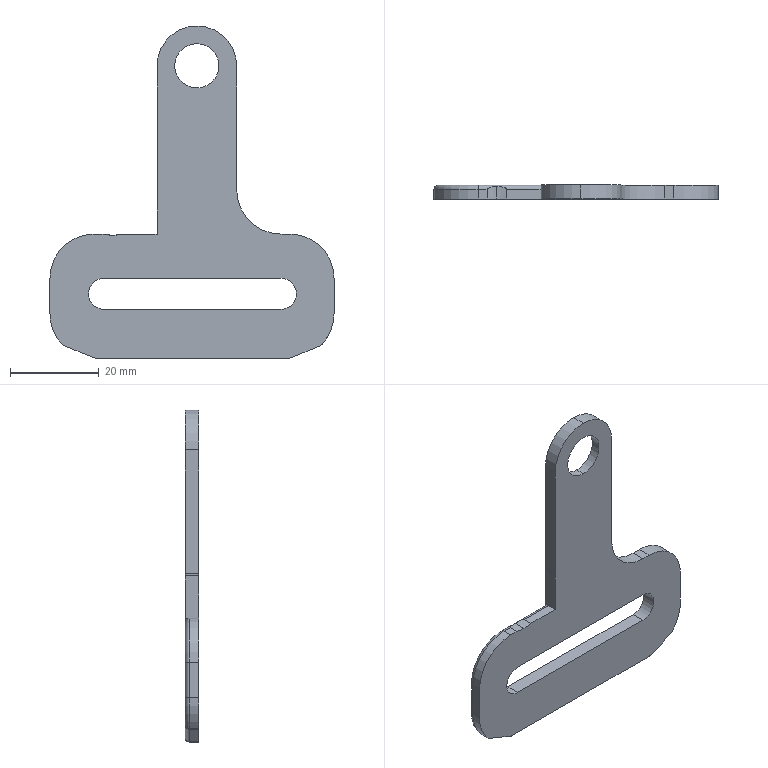Part | SolidWorks | features Fillet 5, ICE 3, Chamfer 1, Extrusion 1, HoleWzd 1 | 1 solid | 44 faces | box 64.199 x 3.15 x 75 mm | volume 6691 mm3 | cylinder 22 | plane 15 | sphere 3 | cone 2 | torus 2 | commonest cylinder face diameters 2 x8 20 x8 7 x2 10 x2 18 x2
STEP:
#1=CARTESIAN_POINT('',(1.,2.15,61.));
#2=VERTEX_POINT('',#1);
#3=CARTESIAN_POINT('',(1.,2.15,71.));
#4=VERTEX_POINT('',#3);
#5=CARTESIAN_POINT('',(1.,2.15,66.));
#6=DIRECTION('',(0.,1.,0.));
#7=DIRECTION('',(0.,0.,1.));
#8=AXIS2_PLACEMENT_3D('',#5,#6,#7);
#9=CIRCLE('',#8,5.);
#10=EDGE_CURVE('',#2,#4,#9,.T.);
#11=ORIENTED_EDGE('',*,*,#10,.F.);
#12=CARTESIAN_POINT('',(1.,3.15,59.5));
#13=VERTEX_POINT('',#12);
#14=CARTESIAN_POINT('',(1.,2.15,61.));
#15=DIRECTION('',(0.,0.5547,-0.8321));
#16=VECTOR('',#15,1000.);
#17=LINE('',#14,#16);
#18=EDGE_CURVE('',#2,#13,#17,.T.);
#19=ORIENTED_EDGE('',*,*,#18,.T.);
#20=CARTESIAN_POINT('',(1.,3.15,72.5));
#21=VERTEX_POINT('',#20);
#22=CARTESIAN_POINT('',(1.,3.15,66.));
#23=DIRECTION('',(0.,-1.,0.));
#24=DIRECTION('',(0.,0.,1.));
#25=AXIS2_PLACEMENT_3D('',#22,#23,#24);
#26=CIRCLE('',#25,6.5);
#27=EDGE_CURVE('',#21,#13,#26,.T.);
#28=ORIENTED_EDGE('',*,*,#27,.F.);
#29=CARTESIAN_POINT('',(1.,2.15,71.));
#30=DIRECTION('',(0.,0.5547,0.8321));
#31=VECTOR('',#30,1000.);
#32=LINE('',#29,#31);
#33=EDGE_CURVE('',#4,#21,#32,.T.);
#34=ORIENTED_EDGE('',*,*,#33,.F.);
#35=EDGE_LOOP('',(#11,#19,#28,#34));
#36=FACE_OUTER_BOUND('',#35,.T.);
#37=CARTESIAN_POINT('',(1.,2.15,66.));
#38=DIRECTION('',(0.,1.,0.));
#39=DIRECTION('',(0.,0.,1.));
#40=AXIS2_PLACEMENT_3D('',#37,#38,#39);
#41=CONICAL_SURFACE('',#40,5.,0.9828);
#42=ADVANCED_FACE('',(#36),#41,.F.);
#43=CARTESIAN_POINT('',(1.,0.,61.));
#44=VERTEX_POINT('',#43);
#45=CARTESIAN_POINT('',(1.,0.,71.));
#46=VERTEX_POINT('',#45);
#47=CARTESIAN_POINT('',(1.,0.,66.));
#48=DIRECTION('',(0.,1.,0.));
#49=DIRECTION('',(0.,0.,1.));
#50=AXIS2_PLACEMENT_3D('',#47,#48,#49);
#51=CIRCLE('',#50,5.);
#52=EDGE_CURVE('',#44,#46,#51,.T.);
#53=ORIENTED_EDGE('',*,*,#52,.F.);
#54=CARTESIAN_POINT('',(1.,3.15,61.));
#55=DIRECTION('',(0.,1.,0.));
#56=VECTOR('',#55,1000.);
#57=LINE('',#54,#56);
#58=EDGE_CURVE('',#44,#2,#57,.T.);
#59=ORIENTED_EDGE('',*,*,#58,.T.);
#60=ORIENTED_EDGE('',*,*,#10,.T.);
#61=CARTESIAN_POINT('',(1.,3.15,71.));
#62=DIRECTION('',(0.,1.,0.));
#63=VECTOR('',#62,1000.);
#64=LINE('',#61,#63);
#65=EDGE_CURVE('',#46,#4,#64,.T.);
#66=ORIENTED_EDGE('',*,*,#65,.F.);
#67=EDGE_LOOP('',(#53,#59,#60,#66));
#68=FACE_OUTER_BOUND('',#67,.T.);
#69=CARTESIAN_POINT('',(1.,3.15,66.));
#70=DIRECTION('',(0.,1.,0.));
#71=DIRECTION('',(0.,0.,1.));
#72=AXIS2_PLACEMENT_3D('',#69,#70,#71);
#73=CYLINDRICAL_SURFACE('',#72,5.);
#74=ADVANCED_FACE('',(#68),#73,.F.);
#75=CARTESIAN_POINT('',(-15.795,2.15,28.));
#76=VERTEX_POINT('',#75);
#77=CARTESIAN_POINT('',(-17.997,2.806,27.755));
#78=VERTEX_POINT('',#77);
#79=CARTESIAN_POINT('',(-15.795,2.15,28.));
#80=CARTESIAN_POINT('',(-15.795,2.202,28.));
#81=CARTESIAN_POINT('',(-15.814,2.252,27.996));
#82=CARTESIAN_POINT('',(-15.87,2.337,27.983));
#83=CARTESIAN_POINT('',(-15.907,2.373,27.975));
#84=CARTESIAN_POINT('',(-16.026,2.468,27.95));
#85=CARTESIAN_POINT('',(-16.117,2.514,27.932));
#86=CARTESIAN_POINT('',(-16.395,2.629,27.882));
#87=CARTESIAN_POINT('',(-16.593,2.676,27.852));
#88=CARTESIAN_POINT('',(-16.988,2.747,27.804));
#89=CARTESIAN_POINT('',(-17.188,2.769,27.785));
#90=CARTESIAN_POINT('',(-17.591,2.799,27.761));
#91=CARTESIAN_POINT('',(-17.794,2.806,27.755));
#92=CARTESIAN_POINT('',(-17.997,2.806,27.755));
#93=B_SPLINE_CURVE_WITH_KNOTS('',3,(#79,#80,#81,#82,#83,#84,#85,#86,#87,#88,#89,#90,#91,#92),.UNSPECIFIED.,.F.,.F.,(4,2,2,2,2,2,4),(0.,0.0001535,0.0003071,0.0006141,0.001228,0.001842,0.002457),.UNSPECIFIED.);
#94=EDGE_CURVE('',#76,#78,#93,.T.);
#95=ORIENTED_EDGE('',*,*,#94,.T.);
#96=CARTESIAN_POINT('',(-17.997,0.,27.755));
#97=VERTEX_POINT('',#96);
#98=CARTESIAN_POINT('',(-17.997,3.15,27.755));
#99=DIRECTION('',(0.,-1.,0.));
#100=VECTOR('',#99,1000.);
#101=LINE('',#98,#100);
#102=EDGE_CURVE('',#78,#97,#101,.T.);
#103=ORIENTED_EDGE('',*,*,#102,.T.);
#104=CARTESIAN_POINT('',(-15.795,0.,28.));
#105=VERTEX_POINT('',#104);
#106=CARTESIAN_POINT('',(-17.997,0.,37.755));
#107=DIRECTION('',(0.,-1.,0.));
#108=DIRECTION('',(0.,0.,-1.));
#109=AXIS2_PLACEMENT_3D('',#106,#107,#108);
#110=CIRCLE('',#109,10.);
#111=EDGE_CURVE('',#97,#105,#110,.T.);
#112=ORIENTED_EDGE('',*,*,#111,.T.);
#113=CARTESIAN_POINT('',(-15.795,3.15,28.));
#114=DIRECTION('',(0.,-1.,0.));
#115=VECTOR('',#114,1000.);
#116=LINE('',#113,#115);
#117=EDGE_CURVE('',#76,#105,#116,.T.);
#118=ORIENTED_EDGE('',*,*,#117,.F.);
#119=EDGE_LOOP('',(#95,#103,#112,#118));
#120=FACE_OUTER_BOUND('',#119,.T.);
#121=CARTESIAN_POINT('',(-17.997,3.15,37.755));
#122=DIRECTION('',(0.,-1.,0.));
#123=DIRECTION('',(0.,0.,-1.));
#124=AXIS2_PLACEMENT_3D('',#121,#122,#123);
#125=CYLINDRICAL_SURFACE('',#124,10.);
#126=ADVANCED_FACE('',(#120),#125,.F.);
#127=CARTESIAN_POINT('',(-8.,0.,66.));
#128=VERTEX_POINT('',#127);
#129=CARTESIAN_POINT('',(1.,0.,75.));
#130=VERTEX_POINT('',#129);
#131=CARTESIAN_POINT('',(1.,0.,66.));
#132=DIRECTION('',(0.,1.,0.));
#133=DIRECTION('',(0.,0.,1.));
#134=AXIS2_PLACEMENT_3D('',#131,#132,#133);
#135=CIRCLE('',#134,9.);
#136=EDGE_CURVE('',#128,#130,#135,.T.);
#137=ORIENTED_EDGE('',*,*,#136,.T.);
#138=CARTESIAN_POINT('',(1.,3.15,75.));
#139=VERTEX_POINT('',#138);
#140=CARTESIAN_POINT('',(1.,0.,75.));
#141=DIRECTION('',(0.,1.,0.));
#142=VECTOR('',#141,1000.);
#143=LINE('',#140,#142);
#144=EDGE_CURVE('',#130,#139,#143,.T.);
#145=ORIENTED_EDGE('',*,*,#144,.T.);
#146=CARTESIAN_POINT('',(-8.,3.15,66.));
#147=VERTEX_POINT('',#146);
#148=CARTESIAN_POINT('',(1.,3.15,66.));
#149=DIRECTION('',(0.,1.,0.));
#150=DIRECTION('',(0.,0.,1.));
#151=AXIS2_PLACEMENT_3D('',#148,#149,#150);
#152=CIRCLE('',#151,9.);
#153=EDGE_CURVE('',#147,#139,#152,.T.);
#154=ORIENTED_EDGE('',*,*,#153,.F.);
#155=CARTESIAN_POINT('',(-8.,0.,66.));
#156=DIRECTION('',(0.,1.,0.));
#157=VECTOR('',#156,1000.);
#158=LINE('',#155,#157);
#159=EDGE_CURVE('',#128,#147,#158,.T.);
#160=ORIENTED_EDGE('',*,*,#159,.F.);
#161=EDGE_LOOP('',(#137,#145,#154,#160));
#162=FACE_OUTER_BOUND('',#161,.T.);
#163=CARTESIAN_POINT('',(1.,0.,66.));
#164=DIRECTION('',(0.,1.,0.));
#165=DIRECTION('',(0.,0.,1.));
#166=AXIS2_PLACEMENT_3D('',#163,#164,#165);
#167=CYLINDRICAL_SURFACE('',#166,9.);
#168=ADVANCED_FACE('',(#162),#167,.T.);
#169=CARTESIAN_POINT('',(-8.,3.15,37.509));
#170=VERTEX_POINT('',#169);
#171=CARTESIAN_POINT('',(-8.,0.,37.509));
#172=VERTEX_POINT('',#171);
#173=CARTESIAN_POINT('',(-8.,3.15,37.509));
#174=DIRECTION('',(0.,-1.,0.));
#175=VECTOR('',#174,1000.);
#176=LINE('',#173,#175);
#177=EDGE_CURVE('',#170,#172,#176,.T.);
#178=ORIENTED_EDGE('',*,*,#177,.F.);
#179=CARTESIAN_POINT('',(-8.,3.15,27.));
#180=VERTEX_POINT('',#179);
#181=CARTESIAN_POINT('',(-8.,3.15,28.));
#182=DIRECTION('',(0.,0.,1.));
#183=VECTOR('',#182,1000.);
#184=LINE('',#181,#183);
#185=EDGE_CURVE('',#180,#170,#184,.T.);
#186=ORIENTED_EDGE('',*,*,#185,.F.);
#187=CARTESIAN_POINT('',(-8.,2.15,28.));
#188=VERTEX_POINT('',#187);
#189=CARTESIAN_POINT('',(-8.,2.15,27.));
#190=DIRECTION('',(1.,0.,0.));
#191=DIRECTION('',(0.,0.,1.));
#192=AXIS2_PLACEMENT_3D('',#189,#190,#191);
#193=CIRCLE('',#192,1.);
#194=EDGE_CURVE('',#180,#188,#193,.T.);
#195=ORIENTED_EDGE('',*,*,#194,.T.);
#196=CARTESIAN_POINT('',(-8.,0.,28.));
#197=VERTEX_POINT('',#196);
#198=CARTESIAN_POINT('',(-8.,0.,28.));
#199=DIRECTION('',(0.,1.,0.));
#200=VECTOR('',#199,1000.);
#201=LINE('',#198,#200);
#202=EDGE_CURVE('',#197,#188,#201,.T.);
#203=ORIENTED_EDGE('',*,*,#202,.F.);
#204=CARTESIAN_POINT('',(-8.,0.,28.));
#205=DIRECTION('',(0.,0.,1.));
#206=VECTOR('',#205,1000.);
#207=LINE('',#204,#206);
#208=EDGE_CURVE('',#197,#172,#207,.T.);
#209=ORIENTED_EDGE('',*,*,#208,.T.);
#210=EDGE_LOOP('',(#178,#186,#195,#203,#209));
#211=FACE_OUTER_BOUND('',#210,.T.);
#212=CARTESIAN_POINT('',(-8.,0.,28.));
#213=DIRECTION('',(-1.,0.,0.));
#214=DIRECTION('',(0.,0.,1.));
#215=AXIS2_PLACEMENT_3D('',#212,#213,#214);
#216=PLANE('',#215);
#217=ADVANCED_FACE('',(#211),#216,.T.);
#218=CARTESIAN_POINT('',(-20.199,2.15,28.));
#219=VERTEX_POINT('',#218);
#220=CARTESIAN_POINT('',(-20.199,0.,28.));
#221=VERTEX_POINT('',#220);
#222=CARTESIAN_POINT('',(-20.199,3.15,28.));
#223=DIRECTION('',(0.,-1.,0.));
#224=VECTOR('',#223,1000.);
#225=LINE('',#222,#224);
#226=EDGE_CURVE('',#219,#221,#225,.T.);
#227=ORIENTED_EDGE('',*,*,#226,.F.);
#228=CARTESIAN_POINT('',(-22.199,2.15,28.));
#229=VERTEX_POINT('',#228);
#230=CARTESIAN_POINT('',(-32.199,2.15,28.));
#231=DIRECTION('',(-1.,0.,0.));
#232=VECTOR('',#231,1000.);
#233=LINE('',#230,#232);
#234=EDGE_CURVE('',#219,#229,#233,.T.);
#235=ORIENTED_EDGE('',*,*,#234,.T.);
#236=CARTESIAN_POINT('',(-22.199,0.,28.));
#237=VERTEX_POINT('',#236);
#238=CARTESIAN_POINT('',(-22.199,0.,28.));
#239=DIRECTION('',(0.,-1.,0.));
#240=VECTOR('',#239,1000.);
#241=LINE('',#238,#240);
#242=EDGE_CURVE('',#229,#237,#241,.T.);
#243=ORIENTED_EDGE('',*,*,#242,.T.);
#244=CARTESIAN_POINT('',(-32.199,0.,28.));
#245=DIRECTION('',(1.,0.,0.));
#246=VECTOR('',#245,1000.);
#247=LINE('',#244,#246);
#248=EDGE_CURVE('',#237,#221,#247,.T.);
#249=ORIENTED_EDGE('',*,*,#248,.T.);
#250=EDGE_LOOP('',(#227,#235,#243,#249));
#251=FACE_OUTER_BOUND('',#250,.T.);
#252=CARTESIAN_POINT('',(-32.199,0.,28.));
#253=DIRECTION('',(0.,0.,1.));
#254=DIRECTION('',(1.,0.,0.));
#255=AXIS2_PLACEMENT_3D('',#252,#253,#254);
#256=PLANE('',#255);
#257=ADVANCED_FACE('',(#251),#256,.T.);
#258=CARTESIAN_POINT('',(-32.199,0.,18.));
#259=VERTEX_POINT('',#258);
#260=CARTESIAN_POINT('',(-32.199,2.15,18.));
#261=VERTEX_POINT('',#260);
#262=CARTESIAN_POINT('',(-32.199,0.,18.));
#263=DIRECTION('',(0.,1.,0.));
#264=VECTOR('',#263,1000.);
#265=LINE('',#262,#264);
#266=EDGE_CURVE('',#259,#261,#265,.T.);
#267=ORIENTED_EDGE('',*,*,#266,.T.);
#268=CARTESIAN_POINT('',(-32.199,2.15,10.));
#269=VERTEX_POINT('',#268);
#270=CARTESIAN_POINT('',(-32.199,2.15,10.));
#271=DIRECTION('',(0.,0.,-1.));
#272=VECTOR('',#271,1000.);
#273=LINE('',#270,#272);
#274=EDGE_CURVE('',#261,#269,#273,.T.);
#275=ORIENTED_EDGE('',*,*,#274,.T.);
#276=CARTESIAN_POINT('',(-32.199,0.,10.));
#277=VERTEX_POINT('',#276);
#278=CARTESIAN_POINT('',(-32.199,0.,10.));
#279=DIRECTION('',(0.,1.,0.));
#280=VECTOR('',#279,1000.);
#281=LINE('',#278,#280);
#282=EDGE_CURVE('',#277,#269,#281,.T.);
#283=ORIENTED_EDGE('',*,*,#282,.F.);
#284=CARTESIAN_POINT('',(-32.199,0.,10.));
#285=DIRECTION('',(0.,0.,1.));
#286=VECTOR('',#285,1000.);
#287=LINE('',#284,#286);
#288=EDGE_CURVE('',#277,#259,#287,.T.);
#289=ORIENTED_EDGE('',*,*,#288,.T.);
#290=EDGE_LOOP('',(#267,#275,#283,#289));
#291=FACE_OUTER_BOUND('',#290,.T.);
#292=CARTESIAN_POINT('',(-32.199,0.,10.));
#293=DIRECTION('',(-1.,0.,0.));
#294=DIRECTION('',(0.,0.,1.));
#295=AXIS2_PLACEMENT_3D('',#292,#293,#294);
#296=PLANE('',#295);
#297=ADVANCED_FACE('',(#291),#296,.T.);
#298=ORIENTED_EDGE('',*,*,#282,.T.);
#299=CARTESIAN_POINT('',(-29.421,2.15,3.083));
#300=VERTEX_POINT('',#299);
#301=CARTESIAN_POINT('',(-22.199,2.15,10.));
#302=DIRECTION('',(0.,-1.,0.));
#303=DIRECTION('',(0.,0.,1.));
#304=AXIS2_PLACEMENT_3D('',#301,#302,#303);
#305=CIRCLE('',#304,10.);
#306=EDGE_CURVE('',#269,#300,#305,.T.);
#307=ORIENTED_EDGE('',*,*,#306,.T.);
#308=CARTESIAN_POINT('',(-29.421,0.,3.083));
#309=VERTEX_POINT('',#308);
#310=CARTESIAN_POINT('',(-29.421,0.,3.083));
#311=DIRECTION('',(0.,-1.,0.));
#312=VECTOR('',#311,1000.);
#313=LINE('',#310,#312);
#314=EDGE_CURVE('',#300,#309,#313,.T.);
#315=ORIENTED_EDGE('',*,*,#314,.T.);
#316=CARTESIAN_POINT('',(-22.199,0.,10.));
#317=DIRECTION('',(0.,1.,0.));
#318=DIRECTION('',(0.,0.,1.));
#319=AXIS2_PLACEMENT_3D('',#316,#317,#318);
#320=CIRCLE('',#319,10.);
#321=EDGE_CURVE('',#309,#277,#320,.T.);
#322=ORIENTED_EDGE('',*,*,#321,.T.);
#323=EDGE_LOOP('',(#298,#307,#315,#322));
#324=FACE_OUTER_BOUND('',#323,.T.);
#325=CARTESIAN_POINT('',(-22.199,0.,10.));
#326=DIRECTION('',(0.,1.,0.));
#327=DIRECTION('',(0.,0.,1.));
#328=AXIS2_PLACEMENT_3D('',#325,#326,#327);
#329=CYLINDRICAL_SURFACE('',#328,10.);
#330=ADVANCED_FACE('',(#324),#329,.T.);
#331=CARTESIAN_POINT('',(-29.081,2.15,2.851));
#332=VERTEX_POINT('',#331);
#333=CARTESIAN_POINT('',(-22.383,2.15,0.07612));
#334=VERTEX_POINT('',#333);
#335=CARTESIAN_POINT('',(-22.199,2.15,0.));
#336=DIRECTION('',(0.9239,0.,-0.3827));
#337=VECTOR('',#336,1000.);
#338=LINE('',#335,#337);
#339=EDGE_CURVE('',#332,#334,#338,.T.);
#340=ORIENTED_EDGE('',*,*,#339,.T.);
#341=CARTESIAN_POINT('',(-22.383,0.,0.07612));
#342=VERTEX_POINT('',#341);
#343=CARTESIAN_POINT('',(-22.383,0.,0.07612));
#344=DIRECTION('',(0.,-1.,0.));
#345=VECTOR('',#344,1000.);
#346=LINE('',#343,#345);
#347=EDGE_CURVE('',#334,#342,#346,.T.);
#348=ORIENTED_EDGE('',*,*,#347,.T.);
#349=CARTESIAN_POINT('',(-29.081,0.,2.851));
#350=VERTEX_POINT('',#349);
#351=CARTESIAN_POINT('',(-22.199,0.,0.));
#352=DIRECTION('',(-0.9239,0.,0.3827));
#353=VECTOR('',#352,1000.);
#354=LINE('',#351,#353);
#355=EDGE_CURVE('',#342,#350,#354,.T.);
#356=ORIENTED_EDGE('',*,*,#355,.T.);
#357=CARTESIAN_POINT('',(-29.081,0.,2.851));
#358=DIRECTION('',(0.,1.,0.));
#359=VECTOR('',#358,1000.);
#360=LINE('',#357,#359);
#361=EDGE_CURVE('',#350,#332,#360,.T.);
#362=ORIENTED_EDGE('',*,*,#361,.T.);
#363=EDGE_LOOP('',(#340,#348,#356,#362));
#364=FACE_OUTER_BOUND('',#363,.T.);
#365=CARTESIAN_POINT('',(-22.199,0.,0.));
#366=DIRECTION('',(-0.3827,0.,-0.9239));
#367=DIRECTION('',(-0.9239,0.,0.3827));
#368=AXIS2_PLACEMENT_3D('',#365,#366,#367);
#369=PLANE('',#368);
#370=ADVANCED_FACE('',(#364),#369,.T.);
#371=CARTESIAN_POINT('',(22.,0.,0.));
#372=VERTEX_POINT('',#371);
#373=CARTESIAN_POINT('',(-22.,0.,0.));
#374=VERTEX_POINT('',#373);
#375=CARTESIAN_POINT('',(22.199,0.,0.));
#376=DIRECTION('',(-1.,0.,0.));
#377=VECTOR('',#376,1000.);
#378=LINE('',#375,#377);
#379=EDGE_CURVE('',#372,#374,#378,.T.);
#380=ORIENTED_EDGE('',*,*,#379,.T.);
#381=CARTESIAN_POINT('',(-22.,2.15,0.));
#382=VERTEX_POINT('',#381);
#383=CARTESIAN_POINT('',(-22.,0.,0.));
#384=DIRECTION('',(0.,1.,0.));
#385=VECTOR('',#384,1000.);
#386=LINE('',#383,#385);
#387=EDGE_CURVE('',#374,#382,#386,.T.);
#388=ORIENTED_EDGE('',*,*,#387,.T.);
#389=CARTESIAN_POINT('',(22.,2.15,0.));
#390=VERTEX_POINT('',#389);
#391=CARTESIAN_POINT('',(22.199,2.15,0.));
#392=DIRECTION('',(1.,0.,0.));
#393=VECTOR('',#392,1000.);
#394=LINE('',#391,#393);
#395=EDGE_CURVE('',#382,#390,#394,.T.);
#396=ORIENTED_EDGE('',*,*,#395,.T.);
#397=CARTESIAN_POINT('',(22.,0.,0.));
#398=DIRECTION('',(0.,-1.,0.));
#399=VECTOR('',#398,1000.);
#400=LINE('',#397,#399);
#401=EDGE_CURVE('',#390,#372,#400,.T.);
#402=ORIENTED_EDGE('',*,*,#401,.T.);
#403=EDGE_LOOP('',(#380,#388,#396,#402));
#404=FACE_OUTER_BOUND('',#403,.T.);
#405=CARTESIAN_POINT('',(22.199,0.,0.));
#406=DIRECTION('',(0.,0.,-1.));
#407=DIRECTION('',(-1.,0.,0.));
#408=AXIS2_PLACEMENT_3D('',#405,#406,#407);
#409=PLANE('',#408);
#410=ADVANCED_FACE('',(#404),#409,.T.);
#411=CARTESIAN_POINT('',(28.925,0.,2.786));
#412=VERTEX_POINT('',#411);
#413=CARTESIAN_POINT('',(22.383,0.,0.07612));
#414=VERTEX_POINT('',#413);
#415=CARTESIAN_POINT('',(28.925,0.,2.786));
#416=DIRECTION('',(-0.9239,0.,-0.3827));
#417=VECTOR('',#416,1000.);
#418=LINE('',#415,#417);
#419=EDGE_CURVE('',#412,#414,#418,.T.);
#420=ORIENTED_EDGE('',*,*,#419,.T.);
#421=CARTESIAN_POINT('',(22.383,2.15,0.07612));
#422=VERTEX_POINT('',#421);
#423=CARTESIAN_POINT('',(22.383,0.,0.07612));
#424=DIRECTION('',(0.,1.,0.));
#425=VECTOR('',#424,1000.);
#426=LINE('',#423,#425);
#427=EDGE_CURVE('',#414,#422,#426,.T.);
#428=ORIENTED_EDGE('',*,*,#427,.T.);
#429=CARTESIAN_POINT('',(28.925,2.15,2.786));
#430=VERTEX_POINT('',#429);
#431=CARTESIAN_POINT('',(28.925,2.15,2.786));
#432=DIRECTION('',(0.9239,0.,0.3827));
#433=VECTOR('',#432,1000.);
#434=LINE('',#431,#433);
#435=EDGE_CURVE('',#422,#430,#434,.T.);
#436=ORIENTED_EDGE('',*,*,#435,.T.);
#437=CARTESIAN_POINT('',(28.925,0.,2.786));
#438=DIRECTION('',(0.,1.,0.));
#439=VECTOR('',#438,1000.);
#440=LINE('',#437,#439);
#441=EDGE_CURVE('',#412,#430,#440,.T.);
#442=ORIENTED_EDGE('',*,*,#441,.F.);
#443=EDGE_LOOP('',(#420,#428,#436,#442));
#444=FACE_OUTER_BOUND('',#443,.T.);
#445=CARTESIAN_POINT('',(28.925,0.,2.786));
#446=DIRECTION('',(0.3827,0.,-0.9239));
#447=DIRECTION('',(-0.9239,0.,-0.3827));
#448=AXIS2_PLACEMENT_3D('',#445,#446,#447);
#449=PLANE('',#448);
#450=ADVANCED_FACE('',(#444),#449,.T.);
#451=ORIENTED_EDGE('',*,*,#441,.T.);
#452=CARTESIAN_POINT('',(30.314,3.15,4.444));
#453=VERTEX_POINT('',#452);
#454=CARTESIAN_POINT('',(28.925,2.15,2.786));
#455=CARTESIAN_POINT('',(28.925,2.258,2.786));
#456=CARTESIAN_POINT('',(28.961,2.358,2.821));
#457=CARTESIAN_POINT('',(29.058,2.525,2.916));
#458=CARTESIAN_POINT('',(29.117,2.592,2.974));
#459=CARTESIAN_POINT('',(29.301,2.773,3.164));
#460=CARTESIAN_POINT('',(29.432,2.86,3.306));
#461=CARTESIAN_POINT('',(29.693,3.003,3.609));
#462=CARTESIAN_POINT('',(29.823,3.056,3.768));
#463=CARTESIAN_POINT('',(30.074,3.13,4.096));
#464=CARTESIAN_POINT('',(30.196,3.15,4.267));
#465=CARTESIAN_POINT('',(30.314,3.15,4.444));
#466=B_SPLINE_CURVE_WITH_KNOTS('',3,(#454,#455,#456,#457,#458,#459,#460,#461,#462,#463,#464,#465),.UNSPECIFIED.,.F.,.F.,(4,2,2,2,2,4),(0.,0.0003194,0.0006387,0.001277,0.001916,0.002555),.UNSPECIFIED.);
#467=EDGE_CURVE('',#430,#453,#466,.T.);
#468=ORIENTED_EDGE('',*,*,#467,.T.);
#469=CARTESIAN_POINT('',(32.,3.15,10.));
#470=VERTEX_POINT('',#469);
#471=CARTESIAN_POINT('',(22.,3.15,10.));
#472=DIRECTION('',(0.,1.,0.));
#473=DIRECTION('',(0.,0.,1.));
#474=AXIS2_PLACEMENT_3D('',#471,#472,#473);
#475=CIRCLE('',#474,10.);
#476=EDGE_CURVE('',#470,#453,#475,.T.);
#477=ORIENTED_EDGE('',*,*,#476,.F.);
#478=CARTESIAN_POINT('',(32.,0.,10.));
#479=VERTEX_POINT('',#478);
#480=CARTESIAN_POINT('',(32.,0.,10.));
#481=DIRECTION('',(0.,1.,0.));
#482=VECTOR('',#481,1000.);
#483=LINE('',#480,#482);
#484=EDGE_CURVE('',#479,#470,#483,.T.);
#485=ORIENTED_EDGE('',*,*,#484,.F.);
#486=CARTESIAN_POINT('',(22.,0.,10.));
#487=DIRECTION('',(0.,1.,0.));
#488=DIRECTION('',(0.,0.,1.));
#489=AXIS2_PLACEMENT_3D('',#486,#487,#488);
#490=CIRCLE('',#489,10.);
#491=EDGE_CURVE('',#479,#412,#490,.T.);
#492=ORIENTED_EDGE('',*,*,#491,.T.);
#493=EDGE_LOOP('',(#451,#468,#477,#485,#492));
#494=FACE_OUTER_BOUND('',#493,.T.);
#495=CARTESIAN_POINT('',(22.,0.,10.));
#496=DIRECTION('',(0.,1.,0.));
#497=DIRECTION('',(0.,0.,1.));
#498=AXIS2_PLACEMENT_3D('',#495,#496,#497);
#499=CYLINDRICAL_SURFACE('',#498,10.);
#500=ADVANCED_FACE('',(#494),#499,.T.);
#501=CARTESIAN_POINT('',(32.,3.15,18.));
#502=VERTEX_POINT('',#501);
#503=CARTESIAN_POINT('',(32.,3.15,28.));
#504=DIRECTION('',(0.,0.,-1.));
#505=VECTOR('',#504,1000.);
#506=LINE('',#503,#505);
#507=EDGE_CURVE('',#502,#470,#506,.T.);
#508=ORIENTED_EDGE('',*,*,#507,.F.);
#509=CARTESIAN_POINT('',(32.,0.,18.));
#510=VERTEX_POINT('',#509);
#511=CARTESIAN_POINT('',(32.,0.,18.));
#512=DIRECTION('',(0.,-1.,0.));
#513=VECTOR('',#512,1000.);
#514=LINE('',#511,#513);
#515=EDGE_CURVE('',#502,#510,#514,.T.);
#516=ORIENTED_EDGE('',*,*,#515,.T.);
#517=CARTESIAN_POINT('',(32.,0.,28.));
#518=DIRECTION('',(0.,0.,-1.));
#519=VECTOR('',#518,1000.);
#520=LINE('',#517,#519);
#521=EDGE_CURVE('',#510,#479,#520,.T.);
#522=ORIENTED_EDGE('',*,*,#521,.T.);
#523=ORIENTED_EDGE('',*,*,#484,.T.);
#524=EDGE_LOOP('',(#508,#516,#522,#523));
#525=FACE_OUTER_BOUND('',#524,.T.);
#526=CARTESIAN_POINT('',(32.,0.,28.));
#527=DIRECTION('',(1.,0.,0.));
#528=DIRECTION('',(0.,0.,-1.));
#529=AXIS2_PLACEMENT_3D('',#526,#527,#528);
#530=PLANE('',#529);
#531=ADVANCED_FACE('',(#525),#530,.T.);
#532=CARTESIAN_POINT('',(20.,0.,28.));
#533=VERTEX_POINT('',#532);
#534=CARTESIAN_POINT('',(22.,0.,28.));
#535=VERTEX_POINT('',#534);
#536=CARTESIAN_POINT('',(10.,0.,28.));
#537=DIRECTION('',(1.,0.,0.));
#538=VECTOR('',#537,1000.);
#539=LINE('',#536,#538);
#540=EDGE_CURVE('',#533,#535,#539,.T.);
#541=ORIENTED_EDGE('',*,*,#540,.T.);
#542=CARTESIAN_POINT('',(22.,3.15,28.));
#543=VERTEX_POINT('',#542);
#544=CARTESIAN_POINT('',(22.,0.,28.));
#545=DIRECTION('',(0.,1.,0.));
#546=VECTOR('',#545,1000.);
#547=LINE('',#544,#546);
#548=EDGE_CURVE('',#535,#543,#547,.T.);
#549=ORIENTED_EDGE('',*,*,#548,.T.);
#550=CARTESIAN_POINT('',(20.,3.15,28.));
#551=VERTEX_POINT('',#550);
#552=CARTESIAN_POINT('',(10.,3.15,28.));
#553=DIRECTION('',(1.,0.,0.));
#554=VECTOR('',#553,1000.);
#555=LINE('',#552,#554);
#556=EDGE_CURVE('',#551,#543,#555,.T.);
#557=ORIENTED_EDGE('',*,*,#556,.F.);
#558=CARTESIAN_POINT('',(20.,0.,28.));
#559=DIRECTION('',(0.,-1.,0.));
#560=VECTOR('',#559,1000.);
#561=LINE('',#558,#560);
#562=EDGE_CURVE('',#551,#533,#561,.T.);
#563=ORIENTED_EDGE('',*,*,#562,.T.);
#564=EDGE_LOOP('',(#541,#549,#557,#563));
#565=FACE_OUTER_BOUND('',#564,.T.);
#566=CARTESIAN_POINT('',(10.,0.,28.));
#567=DIRECTION('',(0.,0.,1.));
#568=DIRECTION('',(1.,0.,0.));
#569=AXIS2_PLACEMENT_3D('',#566,#567,#568);
#570=PLANE('',#569);
#571=ADVANCED_FACE('',(#565),#570,.T.);
#572=CARTESIAN_POINT('',(10.,0.,66.));
#573=VERTEX_POINT('',#572);
#574=CARTESIAN_POINT('',(10.,0.,38.));
#575=VERTEX_POINT('',#574);
#576=CARTESIAN_POINT('',(10.,0.,66.));
#577=DIRECTION('',(0.,0.,-1.));
#578=VECTOR('',#577,1000.);
#579=LINE('',#576,#578);
#580=EDGE_CURVE('',#573,#575,#579,.T.);
#581=ORIENTED_EDGE('',*,*,#580,.T.);
#582=CARTESIAN_POINT('',(10.,3.15,38.));
#583=VERTEX_POINT('',#582);
#584=CARTESIAN_POINT('',(10.,3.15,38.));
#585=DIRECTION('',(0.,1.,0.));
#586=VECTOR('',#585,1000.);
#587=LINE('',#584,#586);
#588=EDGE_CURVE('',#575,#583,#587,.T.);
#589=ORIENTED_EDGE('',*,*,#588,.T.);
#590=CARTESIAN_POINT('',(10.,3.15,66.));
#591=VERTEX_POINT('',#590);
#592=CARTESIAN_POINT('',(10.,3.15,66.));
#593=DIRECTION('',(0.,0.,-1.));
#594=VECTOR('',#593,1000.);
#595=LINE('',#592,#594);
#596=EDGE_CURVE('',#591,#583,#595,.T.);
#597=ORIENTED_EDGE('',*,*,#596,.F.);
#598=CARTESIAN_POINT('',(10.,0.,66.));
#599=DIRECTION('',(0.,1.,0.));
#600=VECTOR('',#599,1000.);
#601=LINE('',#598,#600);
#602=EDGE_CURVE('',#573,#591,#601,.T.);
#603=ORIENTED_EDGE('',*,*,#602,.F.);
#604=EDGE_LOOP('',(#581,#589,#597,#603));
#605=FACE_OUTER_BOUND('',#604,.T.);
#606=CARTESIAN_POINT('',(10.,0.,66.));
#607=DIRECTION('',(1.,0.,0.));
#608=DIRECTION('',(0.,0.,-1.));
#609=AXIS2_PLACEMENT_3D('',#606,#607,#608);
#610=PLANE('',#609);
#611=ADVANCED_FACE('',(#605),#610,.T.);
#612=ORIENTED_EDGE('',*,*,#144,.F.);
#613=CARTESIAN_POINT('',(1.,0.,66.));
#614=DIRECTION('',(0.,1.,0.));
#615=DIRECTION('',(0.,0.,1.));
#616=AXIS2_PLACEMENT_3D('',#613,#614,#615);
#617=CIRCLE('',#616,9.);
#618=EDGE_CURVE('',#130,#573,#617,.T.);
#619=ORIENTED_EDGE('',*,*,#618,.T.);
#620=ORIENTED_EDGE('',*,*,#602,.T.);
#621=CARTESIAN_POINT('',(1.,3.15,66.));
#622=DIRECTION('',(0.,1.,0.));
#623=DIRECTION('',(0.,0.,1.));
#624=AXIS2_PLACEMENT_3D('',#621,#622,#623);
#625=CIRCLE('',#624,9.);
#626=EDGE_CURVE('',#139,#591,#625,.T.);
#627=ORIENTED_EDGE('',*,*,#626,.F.);
#628=EDGE_LOOP('',(#612,#619,#620,#627));
#629=FACE_OUTER_BOUND('',#628,.T.);
#630=CARTESIAN_POINT('',(1.,0.,66.));
#631=DIRECTION('',(0.,1.,0.));
#632=DIRECTION('',(0.,0.,1.));
#633=AXIS2_PLACEMENT_3D('',#630,#631,#632);
#634=CYLINDRICAL_SURFACE('',#633,9.);
#635=ADVANCED_FACE('',(#629),#634,.T.);
#636=CARTESIAN_POINT('',(-8.,3.15,38.));
#637=VERTEX_POINT('',#636);
#638=CARTESIAN_POINT('',(-8.,0.,38.));
#639=VERTEX_POINT('',#638);
#640=CARTESIAN_POINT('',(-8.,3.15,38.));
#641=DIRECTION('',(0.,-1.,0.));
#642=VECTOR('',#641,1000.);
#643=LINE('',#640,#642);
#644=EDGE_CURVE('',#637,#639,#643,.T.);
#645=ORIENTED_EDGE('',*,*,#644,.T.);
#646=CARTESIAN_POINT('',(-8.,0.,28.));
#647=DIRECTION('',(0.,0.,1.));
#648=VECTOR('',#647,1000.);
#649=LINE('',#646,#648);
#650=EDGE_CURVE('',#639,#128,#649,.T.);
#651=ORIENTED_EDGE('',*,*,#650,.T.);
#652=ORIENTED_EDGE('',*,*,#159,.T.);
#653=CARTESIAN_POINT('',(-8.,3.15,28.));
#654=DIRECTION('',(0.,0.,1.));
#655=VECTOR('',#654,1000.);
#656=LINE('',#653,#655);
#657=EDGE_CURVE('',#637,#147,#656,.T.);
#658=ORIENTED_EDGE('',*,*,#657,.F.);
#659=EDGE_LOOP('',(#645,#651,#652,#658));
#660=FACE_OUTER_BOUND('',#659,.T.);
#661=CARTESIAN_POINT('',(-8.,0.,28.));
#662=DIRECTION('',(-1.,0.,0.));
#663=DIRECTION('',(0.,0.,1.));
#664=AXIS2_PLACEMENT_3D('',#661,#662,#663);
#665=PLANE('',#664);
#666=ADVANCED_FACE('',(#660),#665,.T.);
#667=ORIENTED_EDGE('',*,*,#202,.T.);
#668=CARTESIAN_POINT('',(-11.898,2.15,28.));
#669=DIRECTION('',(-1.,0.,0.));
#670=VECTOR('',#669,1000.);
#671=LINE('',#668,#670);
#672=EDGE_CURVE('',#188,#76,#671,.T.);
#673=ORIENTED_EDGE('',*,*,#672,.T.);
#674=ORIENTED_EDGE('',*,*,#117,.T.);
#675=CARTESIAN_POINT('',(-32.199,0.,28.));
#676=DIRECTION('',(1.,0.,0.));
#677=VECTOR('',#676,1000.);
#678=LINE('',#675,#677);
#679=EDGE_CURVE('',#105,#197,#678,.T.);
#680=ORIENTED_EDGE('',*,*,#679,.T.);
#681=EDGE_LOOP('',(#667,#673,#674,#680));
#682=FACE_OUTER_BOUND('',#681,.T.);
#683=CARTESIAN_POINT('',(-32.199,0.,28.));
#684=DIRECTION('',(0.,0.,1.));
#685=DIRECTION('',(1.,0.,0.));
#686=AXIS2_PLACEMENT_3D('',#683,#684,#685);
#687=PLANE('',#686);
#688=ADVANCED_FACE('',(#682),#687,.T.);
#689=CARTESIAN_POINT('',(1.,0.,66.));
#690=DIRECTION('',(0.,1.,0.));
#691=DIRECTION('',(0.,0.,1.));
#692=AXIS2_PLACEMENT_3D('',#689,#690,#691);
#693=CIRCLE('',#692,5.);
#694=EDGE_CURVE('',#46,#44,#693,.T.);
#695=ORIENTED_EDGE('',*,*,#694,.T.);
#696=ORIENTED_EDGE('',*,*,#52,.T.);
#697=EDGE_LOOP('',(#695,#696));
#698=FACE_BOUND('',#697,.T.);
#699=CARTESIAN_POINT('',(-20.,0.,11.));
#700=VERTEX_POINT('',#699);
#701=CARTESIAN_POINT('',(20.,0.,11.));
#702=VERTEX_POINT('',#701);
#703=CARTESIAN_POINT('',(-20.,0.,11.));
#704=DIRECTION('',(1.,0.,0.));
#705=VECTOR('',#704,1000.);
#706=LINE('',#703,#705);
#707=EDGE_CURVE('',#700,#702,#706,.T.);
#708=ORIENTED_EDGE('',*,*,#707,.F.);
#709=CARTESIAN_POINT('',(-20.,0.,18.));
#710=VERTEX_POINT('',#709);
#711=CARTESIAN_POINT('',(-20.,0.,14.5));
#712=DIRECTION('',(0.,-1.,0.));
#713=DIRECTION('',(0.,0.,-1.));
#714=AXIS2_PLACEMENT_3D('',#711,#712,#713);
#715=CIRCLE('',#714,3.5);
#716=EDGE_CURVE('',#710,#700,#715,.T.);
#717=ORIENTED_EDGE('',*,*,#716,.F.);
#718=CARTESIAN_POINT('',(20.,0.,18.));
#719=VERTEX_POINT('',#718);
#720=CARTESIAN_POINT('',(20.,0.,18.));
#721=DIRECTION('',(-1.,0.,0.));
#722=VECTOR('',#721,1000.);
#723=LINE('',#720,#722);
#724=EDGE_CURVE('',#719,#710,#723,.T.);
#725=ORIENTED_EDGE('',*,*,#724,.F.);
#726=CARTESIAN_POINT('',(20.,0.,14.5));
#727=DIRECTION('',(0.,-1.,0.));
#728=DIRECTION('',(0.,0.,-1.));
#729=AXIS2_PLACEMENT_3D('',#726,#727,#728);
#730=CIRCLE('',#729,3.5);
#731=EDGE_CURVE('',#702,#719,#730,.T.);
#732=ORIENTED_EDGE('',*,*,#731,.F.);
#733=EDGE_LOOP('',(#708,#717,#725,#732));
#734=FACE_BOUND('',#733,.T.);
#735=ORIENTED_EDGE('',*,*,#355,.F.);
#736=CARTESIAN_POINT('',(-22.,0.,1.));
#737=DIRECTION('',(0.,-1.,0.));
#738=DIRECTION('',(0.,0.,1.));
#739=AXIS2_PLACEMENT_3D('',#736,#737,#738);
#740=CIRCLE('',#739,1.);
#741=EDGE_CURVE('',#342,#374,#740,.T.);
#742=ORIENTED_EDGE('',*,*,#741,.T.);
#743=ORIENTED_EDGE('',*,*,#379,.F.);
#744=CARTESIAN_POINT('',(22.,0.,1.));
#745=DIRECTION('',(0.,-1.,0.));
#746=DIRECTION('',(0.,0.,1.));
#747=AXIS2_PLACEMENT_3D('',#744,#745,#746);
#748=CIRCLE('',#747,1.);
#749=EDGE_CURVE('',#372,#414,#748,.T.);
#750=ORIENTED_EDGE('',*,*,#749,.T.);
#751=ORIENTED_EDGE('',*,*,#419,.F.);
#752=ORIENTED_EDGE('',*,*,#491,.F.);
#753=ORIENTED_EDGE('',*,*,#521,.F.);
#754=CARTESIAN_POINT('',(22.,0.,18.));
#755=DIRECTION('',(0.,-1.,0.));
#756=DIRECTION('',(0.,0.,1.));
#757=AXIS2_PLACEMENT_3D('',#754,#755,#756);
#758=CIRCLE('',#757,10.);
#759=EDGE_CURVE('',#510,#535,#758,.T.);
#760=ORIENTED_EDGE('',*,*,#759,.T.);
#761=ORIENTED_EDGE('',*,*,#540,.F.);
#762=CARTESIAN_POINT('',(20.,0.,38.));
#763=DIRECTION('',(0.,1.,0.));
#764=DIRECTION('',(0.,0.,1.));
#765=AXIS2_PLACEMENT_3D('',#762,#763,#764);
#766=CIRCLE('',#765,10.);
#767=EDGE_CURVE('',#533,#575,#766,.T.);
#768=ORIENTED_EDGE('',*,*,#767,.T.);
#769=ORIENTED_EDGE('',*,*,#580,.F.);
#770=ORIENTED_EDGE('',*,*,#618,.F.);
#771=ORIENTED_EDGE('',*,*,#136,.F.);
#772=ORIENTED_EDGE('',*,*,#650,.F.);
#773=CARTESIAN_POINT('',(-17.997,0.,37.755));
#774=DIRECTION('',(0.,-1.,0.));
#775=DIRECTION('',(0.,0.,-1.));
#776=AXIS2_PLACEMENT_3D('',#773,#774,#775);
#777=CIRCLE('',#776,10.);
#778=EDGE_CURVE('',#172,#639,#777,.T.);
#779=ORIENTED_EDGE('',*,*,#778,.F.);
#780=ORIENTED_EDGE('',*,*,#208,.F.);
#781=ORIENTED_EDGE('',*,*,#679,.F.);
#782=ORIENTED_EDGE('',*,*,#111,.F.);
#783=CARTESIAN_POINT('',(-17.997,0.,37.755));
#784=DIRECTION('',(0.,-1.,0.));
#785=DIRECTION('',(0.,0.,-1.));
#786=AXIS2_PLACEMENT_3D('',#783,#784,#785);
#787=CIRCLE('',#786,10.);
#788=EDGE_CURVE('',#221,#97,#787,.T.);
#789=ORIENTED_EDGE('',*,*,#788,.F.);
#790=ORIENTED_EDGE('',*,*,#248,.F.);
#791=CARTESIAN_POINT('',(-22.199,0.,18.));
#792=DIRECTION('',(0.,-1.,0.));
#793=DIRECTION('',(0.,0.,1.));
#794=AXIS2_PLACEMENT_3D('',#791,#792,#793);
#795=CIRCLE('',#794,10.);
#796=EDGE_CURVE('',#237,#259,#795,.T.);
#797=ORIENTED_EDGE('',*,*,#796,.T.);
#798=ORIENTED_EDGE('',*,*,#288,.F.);
#799=ORIENTED_EDGE('',*,*,#321,.F.);
#800=CARTESIAN_POINT('',(-28.698,0.,3.775));
#801=DIRECTION('',(0.,-1.,0.));
#802=DIRECTION('',(0.,0.,1.));
#803=AXIS2_PLACEMENT_3D('',#800,#801,#802);
#804=CIRCLE('',#803,1.);
#805=EDGE_CURVE('',#309,#350,#804,.T.);
#806=ORIENTED_EDGE('',*,*,#805,.T.);
#807=EDGE_LOOP('',(#735,#742,#743,#750,#751,#752,#753,#760,#761,#768,#769,#770,#771,#772,#779,#780,#781,#782,#789,#790,#797,#798,#799,#806));
#808=FACE_OUTER_BOUND('',#807,.T.);
#809=CARTESIAN_POINT('',(1.,0.,66.));
#810=DIRECTION('',(0.,1.,0.));
#811=DIRECTION('',(0.,0.,1.));
#812=AXIS2_PLACEMENT_3D('',#809,#810,#811);
#813=PLANE('',#812);
#814=ADVANCED_FACE('',(#698,#734,#808),#813,.F.);
#815=ORIENTED_EDGE('',*,*,#27,.T.);
#816=CARTESIAN_POINT('',(1.,3.15,66.));
#817=DIRECTION('',(0.,-1.,0.));
#818=DIRECTION('',(0.,0.,1.));
#819=AXIS2_PLACEMENT_3D('',#816,#817,#818);
#820=CIRCLE('',#819,6.5);
#821=EDGE_CURVE('',#13,#21,#820,.T.);
#822=ORIENTED_EDGE('',*,*,#821,.T.);
#823=EDGE_LOOP('',(#815,#822));
#824=FACE_BOUND('',#823,.T.);
#825=CARTESIAN_POINT('',(-20.,3.15,18.));
#826=VERTEX_POINT('',#825);
#827=CARTESIAN_POINT('',(-20.,3.15,11.));
#828=VERTEX_POINT('',#827);
#829=CARTESIAN_POINT('',(-20.,3.15,14.5));
#830=DIRECTION('',(0.,-1.,0.));
#831=DIRECTION('',(0.,0.,-1.));
#832=AXIS2_PLACEMENT_3D('',#829,#830,#831);
#833=CIRCLE('',#832,3.5);
#834=EDGE_CURVE('',#826,#828,#833,.T.);
#835=ORIENTED_EDGE('',*,*,#834,.T.);
#836=CARTESIAN_POINT('',(20.,3.15,11.));
#837=VERTEX_POINT('',#836);
#838=CARTESIAN_POINT('',(-20.,3.15,11.));
#839=DIRECTION('',(1.,0.,0.));
#840=VECTOR('',#839,1000.);
#841=LINE('',#838,#840);
#842=EDGE_CURVE('',#828,#837,#841,.T.);
#843=ORIENTED_EDGE('',*,*,#842,.T.);
#844=CARTESIAN_POINT('',(20.,3.15,18.));
#845=VERTEX_POINT('',#844);
#846=CARTESIAN_POINT('',(20.,3.15,14.5));
#847=DIRECTION('',(0.,-1.,0.));
#848=DIRECTION('',(0.,0.,-1.));
#849=AXIS2_PLACEMENT_3D('',#846,#847,#848);
#850=CIRCLE('',#849,3.5);
#851=EDGE_CURVE('',#837,#845,#850,.T.);
#852=ORIENTED_EDGE('',*,*,#851,.T.);
#853=CARTESIAN_POINT('',(20.,3.15,18.));
#854=DIRECTION('',(-1.,0.,0.));
#855=VECTOR('',#854,1000.);
#856=LINE('',#853,#855);
#857=EDGE_CURVE('',#845,#826,#856,.T.);
#858=ORIENTED_EDGE('',*,*,#857,.T.);
#859=EDGE_LOOP('',(#835,#843,#852,#858));
#860=FACE_BOUND('',#859,.T.);
#861=CARTESIAN_POINT('',(-22.199,3.15,27.));
#862=VERTEX_POINT('',#861);
#863=CARTESIAN_POINT('',(1.,3.15,27.));
#864=DIRECTION('',(1.,0.,0.));
#865=VECTOR('',#864,1000.);
#866=LINE('',#863,#865);
#867=EDGE_CURVE('',#862,#180,#866,.T.);
#868=ORIENTED_EDGE('',*,*,#867,.T.);
#869=ORIENTED_EDGE('',*,*,#185,.T.);
#870=CARTESIAN_POINT('',(-17.997,3.15,37.755));
#871=DIRECTION('',(0.,-1.,0.));
#872=DIRECTION('',(0.,0.,-1.));
#873=AXIS2_PLACEMENT_3D('',#870,#871,#872);
#874=CIRCLE('',#873,10.);
#875=EDGE_CURVE('',#170,#637,#874,.T.);
#876=ORIENTED_EDGE('',*,*,#875,.T.);
#877=ORIENTED_EDGE('',*,*,#657,.T.);
#878=ORIENTED_EDGE('',*,*,#153,.T.);
#879=ORIENTED_EDGE('',*,*,#626,.T.);
#880=ORIENTED_EDGE('',*,*,#596,.T.);
#881=CARTESIAN_POINT('',(20.,3.15,38.));
#882=DIRECTION('',(0.,-1.,0.));
#883=DIRECTION('',(0.,0.,1.));
#884=AXIS2_PLACEMENT_3D('',#881,#882,#883);
#885=CIRCLE('',#884,10.);
#886=EDGE_CURVE('',#583,#551,#885,.T.);
#887=ORIENTED_EDGE('',*,*,#886,.T.);
#888=ORIENTED_EDGE('',*,*,#556,.T.);
#889=CARTESIAN_POINT('',(22.,3.15,18.));
#890=DIRECTION('',(0.,1.,0.));
#891=DIRECTION('',(0.,0.,1.));
#892=AXIS2_PLACEMENT_3D('',#889,#890,#891);
#893=CIRCLE('',#892,10.);
#894=EDGE_CURVE('',#543,#502,#893,.T.);
#895=ORIENTED_EDGE('',*,*,#894,.T.);
#896=ORIENTED_EDGE('',*,*,#507,.T.);
#897=ORIENTED_EDGE('',*,*,#476,.T.);
#898=CARTESIAN_POINT('',(22.,3.15,1.));
#899=VERTEX_POINT('',#898);
#900=CARTESIAN_POINT('',(27.056,3.15,3.094));
#901=DIRECTION('',(-0.9239,0.,-0.3827));
#902=VECTOR('',#901,1000.);
#903=LINE('',#900,#902);
#904=EDGE_CURVE('',#453,#899,#903,.T.);
#905=ORIENTED_EDGE('',*,*,#904,.T.);
#906=CARTESIAN_POINT('',(-22.,3.15,1.));
#907=VERTEX_POINT('',#906);
#908=CARTESIAN_POINT('',(1.,3.15,1.));
#909=DIRECTION('',(-1.,0.,0.));
#910=VECTOR('',#909,1000.);
#911=LINE('',#908,#910);
#912=EDGE_CURVE('',#899,#907,#911,.T.);
#913=ORIENTED_EDGE('',*,*,#912,.T.);
#914=CARTESIAN_POINT('',(-28.698,3.15,3.775));
#915=VERTEX_POINT('',#914);
#916=CARTESIAN_POINT('',(-25.349,3.15,2.387));
#917=DIRECTION('',(-0.9239,0.,0.3827));
#918=VECTOR('',#917,1000.);
#919=LINE('',#916,#918);
#920=EDGE_CURVE('',#907,#915,#919,.T.);
#921=ORIENTED_EDGE('',*,*,#920,.T.);
#922=CARTESIAN_POINT('',(-31.199,3.15,10.));
#923=VERTEX_POINT('',#922);
#924=CARTESIAN_POINT('',(-22.199,3.15,10.));
#925=DIRECTION('',(0.,1.,0.));
#926=DIRECTION('',(0.,0.,1.));
#927=AXIS2_PLACEMENT_3D('',#924,#925,#926);
#928=CIRCLE('',#927,9.);
#929=EDGE_CURVE('',#915,#923,#928,.T.);
#930=ORIENTED_EDGE('',*,*,#929,.T.);
#931=CARTESIAN_POINT('',(-31.199,3.15,18.));
#932=VERTEX_POINT('',#931);
#933=CARTESIAN_POINT('',(-31.199,3.15,66.));
#934=DIRECTION('',(0.,0.,1.));
#935=VECTOR('',#934,1000.);
#936=LINE('',#933,#935);
#937=EDGE_CURVE('',#923,#932,#936,.T.);
#938=ORIENTED_EDGE('',*,*,#937,.T.);
#939=CARTESIAN_POINT('',(-22.199,3.15,18.));
#940=DIRECTION('',(0.,1.,0.));
#941=DIRECTION('',(0.,0.,1.));
#942=AXIS2_PLACEMENT_3D('',#939,#940,#941);
#943=CIRCLE('',#942,9.);
#944=EDGE_CURVE('',#932,#862,#943,.T.);
#945=ORIENTED_EDGE('',*,*,#944,.T.);
#946=EDGE_LOOP('',(#868,#869,#876,#877,#878,#879,#880,#887,#888,#895,#896,#897,#905,#913,#921,#930,#938,#945));
#947=FACE_OUTER_BOUND('',#946,.T.);
#948=CARTESIAN_POINT('',(1.,3.15,66.));
#949=DIRECTION('',(0.,1.,0.));
#950=DIRECTION('',(0.,0.,1.));
#951=AXIS2_PLACEMENT_3D('',#948,#949,#950);
#952=PLANE('',#951);
#953=ADVANCED_FACE('',(#824,#860,#947),#952,.T.);
#954=ORIENTED_EDGE('',*,*,#102,.F.);
#955=CARTESIAN_POINT('',(-17.997,2.806,27.755));
#956=CARTESIAN_POINT('',(-18.2,2.806,27.755));
#957=CARTESIAN_POINT('',(-18.402,2.799,27.761));
#958=CARTESIAN_POINT('',(-18.804,2.77,27.785));
#959=CARTESIAN_POINT('',(-19.004,2.747,27.803));
#960=CARTESIAN_POINT('',(-19.402,2.676,27.852));
#961=CARTESIAN_POINT('',(-19.601,2.628,27.882));
#962=CARTESIAN_POINT('',(-19.879,2.513,27.933));
#963=CARTESIAN_POINT('',(-19.97,2.467,27.951));
#964=CARTESIAN_POINT('',(-20.088,2.372,27.976));
#965=CARTESIAN_POINT('',(-20.124,2.336,27.983));
#966=CARTESIAN_POINT('',(-20.18,2.252,27.996));
#967=CARTESIAN_POINT('',(-20.199,2.202,28.));
#968=CARTESIAN_POINT('',(-20.199,2.15,28.));
#969=B_SPLINE_CURVE_WITH_KNOTS('',3,(#955,#956,#957,#958,#959,#960,#961,#962,#963,#964,#965,#966,#967,#968),.UNSPECIFIED.,.F.,.F.,(4,2,2,2,2,2,4),(0.002457,0.003071,0.003686,0.004301,0.004608,0.004762,0.004916),.UNSPECIFIED.);
#970=EDGE_CURVE('',#78,#219,#969,.T.);
#971=ORIENTED_EDGE('',*,*,#970,.T.);
#972=ORIENTED_EDGE('',*,*,#226,.T.);
#973=ORIENTED_EDGE('',*,*,#788,.T.);
#974=EDGE_LOOP('',(#954,#971,#972,#973));
#975=FACE_OUTER_BOUND('',#974,.T.);
#976=CARTESIAN_POINT('',(-17.997,3.15,37.755));
#977=DIRECTION('',(0.,-1.,0.));
#978=DIRECTION('',(0.,0.,-1.));
#979=AXIS2_PLACEMENT_3D('',#976,#977,#978);
#980=CYLINDRICAL_SURFACE('',#979,10.);
#981=ADVANCED_FACE('',(#975),#980,.F.);
#982=ORIENTED_EDGE('',*,*,#778,.T.);
#983=ORIENTED_EDGE('',*,*,#644,.F.);
#984=ORIENTED_EDGE('',*,*,#875,.F.);
#985=ORIENTED_EDGE('',*,*,#177,.T.);
#986=EDGE_LOOP('',(#982,#983,#984,#985));
#987=FACE_OUTER_BOUND('',#986,.T.);
#988=CARTESIAN_POINT('',(-17.997,3.15,37.755));
#989=DIRECTION('',(0.,-1.,0.));
#990=DIRECTION('',(0.,0.,-1.));
#991=AXIS2_PLACEMENT_3D('',#988,#989,#990);
#992=CYLINDRICAL_SURFACE('',#991,10.);
#993=ADVANCED_FACE('',(#987),#992,.F.);
#994=ORIENTED_EDGE('',*,*,#716,.T.);
#995=CARTESIAN_POINT('',(-20.,3.15,11.));
#996=DIRECTION('',(0.,-1.,0.));
#997=VECTOR('',#996,1000.);
#998=LINE('',#995,#997);
#999=EDGE_CURVE('',#828,#700,#998,.T.);
#1000=ORIENTED_EDGE('',*,*,#999,.F.);
#1001=ORIENTED_EDGE('',*,*,#834,.F.);
#1002=CARTESIAN_POINT('',(-20.,3.15,18.));
#1003=DIRECTION('',(0.,-1.,0.));
#1004=VECTOR('',#1003,1000.);
#1005=LINE('',#1002,#1004);
#1006=EDGE_CURVE('',#826,#710,#1005,.T.);
#1007=ORIENTED_EDGE('',*,*,#1006,.T.);
#1008=EDGE_LOOP('',(#994,#1000,#1001,#1007));
#1009=FACE_OUTER_BOUND('',#1008,.T.);
#1010=CARTESIAN_POINT('',(-20.,3.15,14.5));
#1011=DIRECTION('',(0.,-1.,0.));
#1012=DIRECTION('',(0.,0.,-1.));
#1013=AXIS2_PLACEMENT_3D('',#1010,#1011,#1012);
#1014=CYLINDRICAL_SURFACE('',#1013,3.5);
#1015=ADVANCED_FACE('',(#1009),#1014,.F.);
#1016=ORIENTED_EDGE('',*,*,#724,.T.);
#1017=ORIENTED_EDGE('',*,*,#1006,.F.);
#1018=ORIENTED_EDGE('',*,*,#857,.F.);
#1019=CARTESIAN_POINT('',(20.,3.15,18.));
#1020=DIRECTION('',(0.,-1.,0.));
#1021=VECTOR('',#1020,1000.);
#1022=LINE('',#1019,#1021);
#1023=EDGE_CURVE('',#845,#719,#1022,.T.);
#1024=ORIENTED_EDGE('',*,*,#1023,.T.);
#1025=EDGE_LOOP('',(#1016,#1017,#1018,#1024));
#1026=FACE_OUTER_BOUND('',#1025,.T.);
#1027=CARTESIAN_POINT('',(20.,3.15,18.));
#1028=DIRECTION('',(0.,0.,1.));
#1029=DIRECTION('',(1.,0.,0.));
#1030=AXIS2_PLACEMENT_3D('',#1027,#1028,#1029);
#1031=PLANE('',#1030);
#1032=ADVANCED_FACE('',(#1026),#1031,.F.);
#1033=ORIENTED_EDGE('',*,*,#731,.T.);
#1034=ORIENTED_EDGE('',*,*,#1023,.F.);
#1035=ORIENTED_EDGE('',*,*,#851,.F.);
#1036=CARTESIAN_POINT('',(20.,3.15,11.));
#1037=DIRECTION('',(0.,-1.,0.));
#1038=VECTOR('',#1037,1000.);
#1039=LINE('',#1036,#1038);
#1040=EDGE_CURVE('',#837,#702,#1039,.T.);
#1041=ORIENTED_EDGE('',*,*,#1040,.T.);
#1042=EDGE_LOOP('',(#1033,#1034,#1035,#1041));
#1043=FACE_OUTER_BOUND('',#1042,.T.);
#1044=CARTESIAN_POINT('',(20.,3.15,14.5));
#1045=DIRECTION('',(0.,-1.,0.));
#1046=DIRECTION('',(0.,0.,-1.));
#1047=AXIS2_PLACEMENT_3D('',#1044,#1045,#1046);
#1048=CYLINDRICAL_SURFACE('',#1047,3.5);
#1049=ADVANCED_FACE('',(#1043),#1048,.F.);
#1050=ORIENTED_EDGE('',*,*,#707,.T.);
#1051=ORIENTED_EDGE('',*,*,#1040,.F.);
#1052=ORIENTED_EDGE('',*,*,#842,.F.);
#1053=ORIENTED_EDGE('',*,*,#999,.T.);
#1054=EDGE_LOOP('',(#1050,#1051,#1052,#1053));
#1055=FACE_OUTER_BOUND('',#1054,.T.);
#1056=CARTESIAN_POINT('',(-20.,3.15,11.));
#1057=DIRECTION('',(0.,0.,-1.));
#1058=DIRECTION('',(-1.,0.,0.));
#1059=AXIS2_PLACEMENT_3D('',#1056,#1057,#1058);
#1060=PLANE('',#1059);
#1061=ADVANCED_FACE('',(#1055),#1060,.F.);
#1062=ORIENTED_EDGE('',*,*,#58,.F.);
#1063=ORIENTED_EDGE('',*,*,#694,.F.);
#1064=ORIENTED_EDGE('',*,*,#65,.T.);
#1065=CARTESIAN_POINT('',(1.,2.15,66.));
#1066=DIRECTION('',(0.,1.,0.));
#1067=DIRECTION('',(0.,0.,1.));
#1068=AXIS2_PLACEMENT_3D('',#1065,#1066,#1067);
#1069=CIRCLE('',#1068,5.);
#1070=EDGE_CURVE('',#4,#2,#1069,.T.);
#1071=ORIENTED_EDGE('',*,*,#1070,.T.);
#1072=EDGE_LOOP('',(#1062,#1063,#1064,#1071));
#1073=FACE_OUTER_BOUND('',#1072,.T.);
#1074=CARTESIAN_POINT('',(1.,3.15,66.));
#1075=DIRECTION('',(0.,1.,0.));
#1076=DIRECTION('',(0.,0.,1.));
#1077=AXIS2_PLACEMENT_3D('',#1074,#1075,#1076);
#1078=CYLINDRICAL_SURFACE('',#1077,5.);
#1079=ADVANCED_FACE('',(#1073),#1078,.F.);
#1080=ORIENTED_EDGE('',*,*,#759,.F.);
#1081=ORIENTED_EDGE('',*,*,#515,.F.);
#1082=ORIENTED_EDGE('',*,*,#894,.F.);
#1083=ORIENTED_EDGE('',*,*,#548,.F.);
#1084=EDGE_LOOP('',(#1080,#1081,#1082,#1083));
#1085=FACE_OUTER_BOUND('',#1084,.T.);
#1086=CARTESIAN_POINT('',(22.,0.,18.));
#1087=DIRECTION('',(0.,1.,0.));
#1088=DIRECTION('',(0.,0.,1.));
#1089=AXIS2_PLACEMENT_3D('',#1086,#1087,#1088);
#1090=CYLINDRICAL_SURFACE('',#1089,10.);
#1091=ADVANCED_FACE('',(#1085),#1090,.T.);
#1092=ORIENTED_EDGE('',*,*,#767,.F.);
#1093=ORIENTED_EDGE('',*,*,#562,.F.);
#1094=ORIENTED_EDGE('',*,*,#886,.F.);
#1095=ORIENTED_EDGE('',*,*,#588,.F.);
#1096=EDGE_LOOP('',(#1092,#1093,#1094,#1095));
#1097=FACE_OUTER_BOUND('',#1096,.T.);
#1098=CARTESIAN_POINT('',(20.,0.,38.));
#1099=DIRECTION('',(0.,-1.,0.));
#1100=DIRECTION('',(0.,0.,-1.));
#1101=AXIS2_PLACEMENT_3D('',#1098,#1099,#1100);
#1102=CYLINDRICAL_SURFACE('',#1101,10.);
#1103=ADVANCED_FACE('',(#1097),#1102,.F.);
#1104=ORIENTED_EDGE('',*,*,#242,.F.);
#1105=CARTESIAN_POINT('',(-22.199,2.15,18.));
#1106=DIRECTION('',(0.,-1.,0.));
#1107=DIRECTION('',(0.,0.,1.));
#1108=AXIS2_PLACEMENT_3D('',#1105,#1106,#1107);
#1109=CIRCLE('',#1108,10.);
#1110=EDGE_CURVE('',#229,#261,#1109,.T.);
#1111=ORIENTED_EDGE('',*,*,#1110,.T.);
#1112=ORIENTED_EDGE('',*,*,#266,.F.);
#1113=ORIENTED_EDGE('',*,*,#796,.F.);
#1114=EDGE_LOOP('',(#1104,#1111,#1112,#1113));
#1115=FACE_OUTER_BOUND('',#1114,.T.);
#1116=CARTESIAN_POINT('',(-22.199,0.,18.));
#1117=DIRECTION('',(0.,1.,0.));
#1118=DIRECTION('',(0.,0.,1.));
#1119=AXIS2_PLACEMENT_3D('',#1116,#1117,#1118);
#1120=CYLINDRICAL_SURFACE('',#1119,10.);
#1121=ADVANCED_FACE('',(#1115),#1120,.T.);
#1122=ORIENTED_EDGE('',*,*,#18,.F.);
#1123=ORIENTED_EDGE('',*,*,#1070,.F.);
#1124=ORIENTED_EDGE('',*,*,#33,.T.);
#1125=ORIENTED_EDGE('',*,*,#821,.F.);
#1126=EDGE_LOOP('',(#1122,#1123,#1124,#1125));
#1127=FACE_OUTER_BOUND('',#1126,.T.);
#1128=CARTESIAN_POINT('',(1.,2.15,66.));
#1129=DIRECTION('',(0.,1.,0.));
#1130=DIRECTION('',(0.,0.,1.));
#1131=AXIS2_PLACEMENT_3D('',#1128,#1129,#1130);
#1132=CONICAL_SURFACE('',#1131,5.,0.9828);
#1133=ADVANCED_FACE('',(#1127),#1132,.F.);
#1134=ORIENTED_EDGE('',*,*,#435,.F.);
#1135=CARTESIAN_POINT('',(22.,2.15,1.));
#1136=DIRECTION('',(0.9239,0.,0.3827));
#1137=DIRECTION('',(-0.3827,0.,0.9239));
#1138=AXIS2_PLACEMENT_3D('',#1135,#1136,#1137);
#1139=CIRCLE('',#1138,1.);
#1140=EDGE_CURVE('',#422,#899,#1139,.T.);
#1141=ORIENTED_EDGE('',*,*,#1140,.T.);
#1142=ORIENTED_EDGE('',*,*,#904,.F.);
#1143=ORIENTED_EDGE('',*,*,#467,.F.);
#1144=EDGE_LOOP('',(#1134,#1141,#1142,#1143));
#1145=FACE_OUTER_BOUND('',#1144,.T.);
#1146=CARTESIAN_POINT('',(27.056,2.15,3.094));
#1147=DIRECTION('',(-0.9239,0.,-0.3827));
#1148=DIRECTION('',(-0.3827,0.,0.9239));
#1149=AXIS2_PLACEMENT_3D('',#1146,#1147,#1148);
#1150=CYLINDRICAL_SURFACE('',#1149,1.);
#1151=ADVANCED_FACE('',(#1145),#1150,.T.);
#1152=CARTESIAN_POINT('',(22.,2.15,1.));
#1153=DIRECTION('',(0.,1.,0.));
#1154=DIRECTION('',(0.,0.,1.));
#1155=AXIS2_PLACEMENT_3D('',#1152,#1153,#1154);
#1156=CIRCLE('',#1155,1.);
#1157=EDGE_CURVE('',#422,#390,#1156,.T.);
#1158=ORIENTED_EDGE('',*,*,#1157,.F.);
#1159=ORIENTED_EDGE('',*,*,#427,.F.);
#1160=ORIENTED_EDGE('',*,*,#749,.F.);
#1161=ORIENTED_EDGE('',*,*,#401,.F.);
#1162=EDGE_LOOP('',(#1158,#1159,#1160,#1161));
#1163=FACE_OUTER_BOUND('',#1162,.T.);
#1164=CARTESIAN_POINT('',(22.,0.,1.));
#1165=DIRECTION('',(0.,1.,0.));
#1166=DIRECTION('',(0.,0.,1.));
#1167=AXIS2_PLACEMENT_3D('',#1164,#1165,#1166);
#1168=CYLINDRICAL_SURFACE('',#1167,1.);
#1169=ADVANCED_FACE('',(#1163),#1168,.T.);
#1170=ORIENTED_EDGE('',*,*,#1140,.F.);
#1171=ORIENTED_EDGE('',*,*,#1157,.T.);
#1172=CARTESIAN_POINT('',(22.,2.15,1.));
#1173=DIRECTION('',(-1.,0.,0.));
#1174=DIRECTION('',(0.,0.,1.));
#1175=AXIS2_PLACEMENT_3D('',#1172,#1173,#1174);
#1176=CIRCLE('',#1175,1.);
#1177=EDGE_CURVE('',#899,#390,#1176,.T.);
#1178=ORIENTED_EDGE('',*,*,#1177,.F.);
#1179=EDGE_LOOP('',(#1170,#1171,#1178));
#1180=FACE_OUTER_BOUND('',#1179,.T.);
#1181=CARTESIAN_POINT('',(22.,2.15,1.));
#1182=DIRECTION('',(0.,1.,0.));
#1183=DIRECTION('',(-1.,0.,0.));
#1184=AXIS2_PLACEMENT_3D('',#1181,#1182,#1183);
#1185=SPHERICAL_SURFACE('',#1184,1.);
#1186=ADVANCED_FACE('',(#1180),#1185,.T.);
#1187=ORIENTED_EDGE('',*,*,#395,.F.);
#1188=CARTESIAN_POINT('',(-22.,2.15,1.));
#1189=DIRECTION('',(1.,0.,0.));
#1190=DIRECTION('',(0.,0.,1.));
#1191=AXIS2_PLACEMENT_3D('',#1188,#1189,#1190);
#1192=CIRCLE('',#1191,1.);
#1193=EDGE_CURVE('',#382,#907,#1192,.T.);
#1194=ORIENTED_EDGE('',*,*,#1193,.T.);
#1195=ORIENTED_EDGE('',*,*,#912,.F.);
#1196=ORIENTED_EDGE('',*,*,#1177,.T.);
#1197=EDGE_LOOP('',(#1187,#1194,#1195,#1196));
#1198=FACE_OUTER_BOUND('',#1197,.T.);
#1199=CARTESIAN_POINT('',(1.,2.15,1.));
#1200=DIRECTION('',(-1.,0.,0.));
#1201=DIRECTION('',(0.,0.,1.));
#1202=AXIS2_PLACEMENT_3D('',#1199,#1200,#1201);
#1203=CYLINDRICAL_SURFACE('',#1202,1.);
#1204=ADVANCED_FACE('',(#1198),#1203,.T.);
#1205=ORIENTED_EDGE('',*,*,#314,.F.);
#1206=CARTESIAN_POINT('',(-28.698,2.15,3.775));
#1207=DIRECTION('',(0.,-1.,0.));
#1208=DIRECTION('',(0.,0.,1.));
#1209=AXIS2_PLACEMENT_3D('',#1206,#1207,#1208);
#1210=CIRCLE('',#1209,1.);
#1211=EDGE_CURVE('',#300,#332,#1210,.T.);
#1212=ORIENTED_EDGE('',*,*,#1211,.T.);
#1213=ORIENTED_EDGE('',*,*,#361,.F.);
#1214=ORIENTED_EDGE('',*,*,#805,.F.);
#1215=EDGE_LOOP('',(#1205,#1212,#1213,#1214));
#1216=FACE_OUTER_BOUND('',#1215,.T.);
#1217=CARTESIAN_POINT('',(-28.698,0.,3.775));
#1218=DIRECTION('',(0.,1.,0.));
#1219=DIRECTION('',(0.,0.,1.));
#1220=AXIS2_PLACEMENT_3D('',#1217,#1218,#1219);
#1221=CYLINDRICAL_SURFACE('',#1220,1.);
#1222=ADVANCED_FACE('',(#1216),#1221,.T.);
#1223=ORIENTED_EDGE('',*,*,#194,.F.);
#1224=ORIENTED_EDGE('',*,*,#867,.F.);
#1225=CARTESIAN_POINT('',(-22.199,2.15,27.));
#1226=DIRECTION('',(-1.,0.,0.));
#1227=DIRECTION('',(0.,0.,1.));
#1228=AXIS2_PLACEMENT_3D('',#1225,#1226,#1227);
#1229=CIRCLE('',#1228,1.);
#1230=EDGE_CURVE('',#229,#862,#1229,.T.);
#1231=ORIENTED_EDGE('',*,*,#1230,.F.);
#1232=ORIENTED_EDGE('',*,*,#234,.F.);
#1233=ORIENTED_EDGE('',*,*,#970,.F.);
#1234=ORIENTED_EDGE('',*,*,#94,.F.);
#1235=ORIENTED_EDGE('',*,*,#672,.F.);
#1236=EDGE_LOOP('',(#1223,#1224,#1231,#1232,#1233,#1234,#1235));
#1237=FACE_OUTER_BOUND('',#1236,.T.);
#1238=CARTESIAN_POINT('',(1.,2.15,27.));
#1239=DIRECTION('',(1.,0.,0.));
#1240=DIRECTION('',(0.,0.,-1.));
#1241=AXIS2_PLACEMENT_3D('',#1238,#1239,#1240);
#1242=CYLINDRICAL_SURFACE('',#1241,1.);
#1243=ADVANCED_FACE('',(#1237),#1242,.T.);
#1244=ORIENTED_EDGE('',*,*,#1230,.T.);
#1245=ORIENTED_EDGE('',*,*,#944,.F.);
#1246=CARTESIAN_POINT('',(-31.199,2.15,18.));
#1247=DIRECTION('',(0.,0.,-1.));
#1248=DIRECTION('',(-1.,0.,0.));
#1249=AXIS2_PLACEMENT_3D('',#1246,#1247,#1248);
#1250=CIRCLE('',#1249,1.);
#1251=EDGE_CURVE('',#261,#932,#1250,.T.);
#1252=ORIENTED_EDGE('',*,*,#1251,.F.);
#1253=ORIENTED_EDGE('',*,*,#1110,.F.);
#1254=EDGE_LOOP('',(#1244,#1245,#1252,#1253));
#1255=FACE_OUTER_BOUND('',#1254,.T.);
#1256=CARTESIAN_POINT('',(-22.199,2.15,18.));
#1257=DIRECTION('',(0.,1.,0.));
#1258=DIRECTION('',(0.,0.,1.));
#1259=AXIS2_PLACEMENT_3D('',#1256,#1257,#1258);
#1260=TOROIDAL_SURFACE('',#1259,9.,1.);
#1261=ADVANCED_FACE('',(#1255),#1260,.T.);
#1262=ORIENTED_EDGE('',*,*,#1251,.T.);
#1263=ORIENTED_EDGE('',*,*,#937,.F.);
#1264=CARTESIAN_POINT('',(-31.199,2.15,10.));
#1265=DIRECTION('',(0.,0.,-1.));
#1266=DIRECTION('',(-1.,0.,0.));
#1267=AXIS2_PLACEMENT_3D('',#1264,#1265,#1266);
#1268=CIRCLE('',#1267,1.);
#1269=EDGE_CURVE('',#269,#923,#1268,.T.);
#1270=ORIENTED_EDGE('',*,*,#1269,.F.);
#1271=ORIENTED_EDGE('',*,*,#274,.F.);
#1272=EDGE_LOOP('',(#1262,#1263,#1270,#1271));
#1273=FACE_OUTER_BOUND('',#1272,.T.);
#1274=CARTESIAN_POINT('',(-31.199,2.15,66.));
#1275=DIRECTION('',(0.,0.,1.));
#1276=DIRECTION('',(1.,0.,0.));
#1277=AXIS2_PLACEMENT_3D('',#1274,#1275,#1276);
#1278=CYLINDRICAL_SURFACE('',#1277,1.);
#1279=ADVANCED_FACE('',(#1273),#1278,.T.);
#1280=CARTESIAN_POINT('',(-28.698,2.15,3.775));
#1281=DIRECTION('',(0.6917,0.,-0.7222));
#1282=DIRECTION('',(-0.7222,0.,-0.6917));
#1283=AXIS2_PLACEMENT_3D('',#1280,#1281,#1282);
#1284=CIRCLE('',#1283,1.);
#1285=EDGE_CURVE('',#300,#915,#1284,.T.);
#1286=ORIENTED_EDGE('',*,*,#1285,.F.);
#1287=ORIENTED_EDGE('',*,*,#306,.F.);
#1288=ORIENTED_EDGE('',*,*,#1269,.T.);
#1289=ORIENTED_EDGE('',*,*,#929,.F.);
#1290=EDGE_LOOP('',(#1286,#1287,#1288,#1289));
#1291=FACE_OUTER_BOUND('',#1290,.T.);
#1292=CARTESIAN_POINT('',(-22.199,2.15,10.));
#1293=DIRECTION('',(0.,1.,0.));
#1294=DIRECTION('',(0.,0.,1.));
#1295=AXIS2_PLACEMENT_3D('',#1292,#1293,#1294);
#1296=TOROIDAL_SURFACE('',#1295,9.,1.);
#1297=ADVANCED_FACE('',(#1291),#1296,.T.);
#1298=ORIENTED_EDGE('',*,*,#1211,.F.);
#1299=ORIENTED_EDGE('',*,*,#1285,.T.);
#1300=CARTESIAN_POINT('',(-28.698,2.15,3.775));
#1301=DIRECTION('',(0.9239,0.,-0.3827));
#1302=DIRECTION('',(-0.3827,0.,-0.9239));
#1303=AXIS2_PLACEMENT_3D('',#1300,#1301,#1302);
#1304=CIRCLE('',#1303,1.);
#1305=EDGE_CURVE('',#332,#915,#1304,.T.);
#1306=ORIENTED_EDGE('',*,*,#1305,.F.);
#1307=EDGE_LOOP('',(#1298,#1299,#1306));
#1308=FACE_OUTER_BOUND('',#1307,.T.);
#1309=CARTESIAN_POINT('',(-28.698,2.15,3.775));
#1310=DIRECTION('',(1.,0.,0.));
#1311=DIRECTION('',(0.,0.,1.));
#1312=AXIS2_PLACEMENT_3D('',#1309,#1310,#1311);
#1313=SPHERICAL_SURFACE('',#1312,1.);
#1314=ADVANCED_FACE('',(#1308),#1313,.T.);
#1315=ORIENTED_EDGE('',*,*,#1305,.T.);
#1316=ORIENTED_EDGE('',*,*,#920,.F.);
#1317=CARTESIAN_POINT('',(-22.,2.15,1.));
#1318=DIRECTION('',(0.9239,0.,-0.3827));
#1319=DIRECTION('',(-0.3827,0.,-0.9239));
#1320=AXIS2_PLACEMENT_3D('',#1317,#1318,#1319);
#1321=CIRCLE('',#1320,1.);
#1322=EDGE_CURVE('',#334,#907,#1321,.T.);
#1323=ORIENTED_EDGE('',*,*,#1322,.F.);
#1324=ORIENTED_EDGE('',*,*,#339,.F.);
#1325=EDGE_LOOP('',(#1315,#1316,#1323,#1324));
#1326=FACE_OUTER_BOUND('',#1325,.T.);
#1327=CARTESIAN_POINT('',(-25.349,2.15,2.387));
#1328=DIRECTION('',(-0.9239,0.,0.3827));
#1329=DIRECTION('',(0.3827,0.,0.9239));
#1330=AXIS2_PLACEMENT_3D('',#1327,#1328,#1329);
#1331=CYLINDRICAL_SURFACE('',#1330,1.);
#1332=ADVANCED_FACE('',(#1326),#1331,.T.);
#1333=ORIENTED_EDGE('',*,*,#1322,.T.);
#1334=ORIENTED_EDGE('',*,*,#1193,.F.);
#1335=CARTESIAN_POINT('',(-22.,2.15,1.));
#1336=DIRECTION('',(0.,-1.,0.));
#1337=DIRECTION('',(0.,0.,-1.));
#1338=AXIS2_PLACEMENT_3D('',#1335,#1336,#1337);
#1339=CIRCLE('',#1338,1.);
#1340=EDGE_CURVE('',#334,#382,#1339,.T.);
#1341=ORIENTED_EDGE('',*,*,#1340,.F.);
#1342=EDGE_LOOP('',(#1333,#1334,#1341));
#1343=FACE_OUTER_BOUND('',#1342,.T.);
#1344=CARTESIAN_POINT('',(-22.,2.15,1.));
#1345=DIRECTION('',(0.,1.,0.));
#1346=DIRECTION('',(-0.9239,0.,0.3827));
#1347=AXIS2_PLACEMENT_3D('',#1344,#1345,#1346);
#1348=SPHERICAL_SURFACE('',#1347,1.);
#1349=ADVANCED_FACE('',(#1343),#1348,.T.);
#1350=ORIENTED_EDGE('',*,*,#741,.F.);
#1351=ORIENTED_EDGE('',*,*,#347,.F.);
#1352=ORIENTED_EDGE('',*,*,#1340,.T.);
#1353=ORIENTED_EDGE('',*,*,#387,.F.);
#1354=EDGE_LOOP('',(#1350,#1351,#1352,#1353));
#1355=FACE_OUTER_BOUND('',#1354,.T.);
#1356=CARTESIAN_POINT('',(-22.,0.,1.));
#1357=DIRECTION('',(0.,1.,0.));
#1358=DIRECTION('',(0.,0.,1.));
#1359=AXIS2_PLACEMENT_3D('',#1356,#1357,#1358);
#1360=CYLINDRICAL_SURFACE('',#1359,1.);
#1361=ADVANCED_FACE('',(#1355),#1360,.T.);
#1362=CLOSED_SHELL('',(#42,#74,#126,#168,#217,#257,#297,#330,#370,#410,#450,#500,#531,#571,#611,#635,#666,#688,#814,#953,#981,#993,#1015,#1032,#1049,#1061,#1079,#1091,#1103,#1121,#1133,#1151,#1169,#1186,#1204,#1222,#1243,#1261,#1279,#1297,#1314,#1332,#1349,#1361));
#1363=MANIFOLD_SOLID_BREP('',#1362);
#1364=CARTESIAN_POINT('',(0.,0.,0.));
#1365=DIRECTION('',(0.,0.,1.));
#1366=DIRECTION('',(1.,0.,0.));
#1367=AXIS2_PLACEMENT_3D('',#1364,#1365,#1366);
#1368=(LENGTH_UNIT()NAMED_UNIT(*)SI_UNIT(.MILLI.,.METRE.));
#1369=UNCERTAINTY_MEASURE_WITH_UNIT(LENGTH_MEASURE(0.00001),#1368,'','');
#1370=(NAMED_UNIT(*)PLANE_ANGLE_UNIT()SI_UNIT($,.RADIAN.));
#1371=(NAMED_UNIT(*)SI_UNIT($,.STERADIAN.)SOLID_ANGLE_UNIT());
#1372=(GEOMETRIC_REPRESENTATION_CONTEXT(3)GLOBAL_UNCERTAINTY_ASSIGNED_CONTEXT((#1369))GLOBAL_UNIT_ASSIGNED_CONTEXT((#1368,#1370,#1371))REPRESENTATION_CONTEXT('',''));
#1373=ADVANCED_BREP_SHAPE_REPRESENTATION('',(#1363,#1367),#1372);